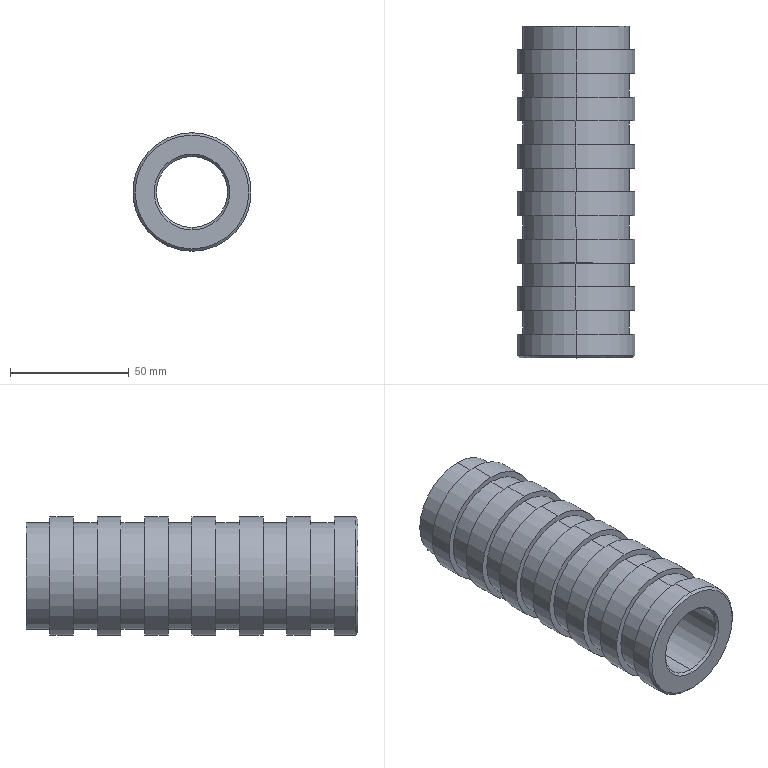Part | SolidWorks | features Revolution 1 | 1 solid | 49 faces | box 50 x 140 x 50 mm | volume 149689 mm3 | cylinder 30 | plane 15 | cone 4 | commonest cylinder face diameters 45 x14 50 x14 30 x2
STEP:
#1=CARTESIAN_POINT('',(0.,-230.,25.));
#2=VERTEX_POINT('',#1);
#3=CARTESIAN_POINT('',(0.,-230.,-25.));
#4=VERTEX_POINT('',#3);
#5=CARTESIAN_POINT('',(0.,-230.,0.));
#6=DIRECTION('',(0.,1.,0.));
#7=DIRECTION('',(0.,0.,1.));
#8=AXIS2_PLACEMENT_3D('',#5,#6,#7);
#9=CIRCLE('',#8,25.);
#10=EDGE_CURVE('',#2,#4,#9,.T.);
#11=ORIENTED_EDGE('',*,*,#10,.T.);
#12=CARTESIAN_POINT('',(0.,-220.,-25.));
#13=VERTEX_POINT('',#12);
#14=CARTESIAN_POINT('',(0.,-290.,-25.));
#15=DIRECTION('',(0.,1.,0.));
#16=VECTOR('',#15,1000.);
#17=LINE('',#14,#16);
#18=EDGE_CURVE('',#4,#13,#17,.T.);
#19=ORIENTED_EDGE('',*,*,#18,.T.);
#20=CARTESIAN_POINT('',(0.,-220.,25.));
#21=VERTEX_POINT('',#20);
#22=CARTESIAN_POINT('',(0.,-220.,0.));
#23=DIRECTION('',(0.,1.,0.));
#24=DIRECTION('',(0.,0.,1.));
#25=AXIS2_PLACEMENT_3D('',#22,#23,#24);
#26=CIRCLE('',#25,25.);
#27=EDGE_CURVE('',#21,#13,#26,.T.);
#28=ORIENTED_EDGE('',*,*,#27,.F.);
#29=CARTESIAN_POINT('',(0.,-290.,25.));
#30=DIRECTION('',(0.,1.,0.));
#31=VECTOR('',#30,1000.);
#32=LINE('',#29,#31);
#33=EDGE_CURVE('',#2,#21,#32,.T.);
#34=ORIENTED_EDGE('',*,*,#33,.F.);
#35=EDGE_LOOP('',(#11,#19,#28,#34));
#36=FACE_OUTER_BOUND('',#35,.T.);
#37=CARTESIAN_POINT('',(0.,-290.,0.));
#38=DIRECTION('',(0.,1.,0.));
#39=DIRECTION('',(0.,0.,1.));
#40=AXIS2_PLACEMENT_3D('',#37,#38,#39);
#41=CYLINDRICAL_SURFACE('',#40,25.);
#42=ADVANCED_FACE('',(#36),#41,.T.);
#43=CARTESIAN_POINT('',(0.,-240.,22.5));
#44=VERTEX_POINT('',#43);
#45=CARTESIAN_POINT('',(0.,-240.,-22.5));
#46=VERTEX_POINT('',#45);
#47=CARTESIAN_POINT('',(0.,-240.,0.));
#48=DIRECTION('',(0.,1.,0.));
#49=DIRECTION('',(0.,0.,1.));
#50=AXIS2_PLACEMENT_3D('',#47,#48,#49);
#51=CIRCLE('',#50,22.5);
#52=EDGE_CURVE('',#44,#46,#51,.T.);
#53=ORIENTED_EDGE('',*,*,#52,.T.);
#54=CARTESIAN_POINT('',(0.,-230.,-22.5));
#55=VERTEX_POINT('',#54);
#56=CARTESIAN_POINT('',(0.,-290.,-22.5));
#57=DIRECTION('',(0.,1.,0.));
#58=VECTOR('',#57,1000.);
#59=LINE('',#56,#58);
#60=EDGE_CURVE('',#46,#55,#59,.T.);
#61=ORIENTED_EDGE('',*,*,#60,.T.);
#62=CARTESIAN_POINT('',(0.,-230.,22.5));
#63=VERTEX_POINT('',#62);
#64=CARTESIAN_POINT('',(0.,-230.,0.));
#65=DIRECTION('',(0.,1.,0.));
#66=DIRECTION('',(0.,0.,1.));
#67=AXIS2_PLACEMENT_3D('',#64,#65,#66);
#68=CIRCLE('',#67,22.5);
#69=EDGE_CURVE('',#63,#55,#68,.T.);
#70=ORIENTED_EDGE('',*,*,#69,.F.);
#71=CARTESIAN_POINT('',(0.,-290.,22.5));
#72=DIRECTION('',(0.,1.,0.));
#73=VECTOR('',#72,1000.);
#74=LINE('',#71,#73);
#75=EDGE_CURVE('',#44,#63,#74,.T.);
#76=ORIENTED_EDGE('',*,*,#75,.F.);
#77=EDGE_LOOP('',(#53,#61,#70,#76));
#78=FACE_OUTER_BOUND('',#77,.T.);
#79=CARTESIAN_POINT('',(0.,-290.,0.));
#80=DIRECTION('',(0.,1.,0.));
#81=DIRECTION('',(0.,0.,1.));
#82=AXIS2_PLACEMENT_3D('',#79,#80,#81);
#83=CYLINDRICAL_SURFACE('',#82,22.5);
#84=ADVANCED_FACE('',(#78),#83,.T.);
#85=CARTESIAN_POINT('',(0.,-250.,25.));
#86=VERTEX_POINT('',#85);
#87=CARTESIAN_POINT('',(0.,-250.,-25.));
#88=VERTEX_POINT('',#87);
#89=CARTESIAN_POINT('',(0.,-250.,0.));
#90=DIRECTION('',(0.,1.,0.));
#91=DIRECTION('',(0.,0.,1.));
#92=AXIS2_PLACEMENT_3D('',#89,#90,#91);
#93=CIRCLE('',#92,25.);
#94=EDGE_CURVE('',#86,#88,#93,.T.);
#95=ORIENTED_EDGE('',*,*,#94,.T.);
#96=CARTESIAN_POINT('',(0.,-240.,-25.));
#97=VERTEX_POINT('',#96);
#98=CARTESIAN_POINT('',(0.,-290.,-25.));
#99=DIRECTION('',(0.,1.,0.));
#100=VECTOR('',#99,1000.);
#101=LINE('',#98,#100);
#102=EDGE_CURVE('',#88,#97,#101,.T.);
#103=ORIENTED_EDGE('',*,*,#102,.T.);
#104=CARTESIAN_POINT('',(0.,-240.,25.));
#105=VERTEX_POINT('',#104);
#106=CARTESIAN_POINT('',(0.,-240.,0.));
#107=DIRECTION('',(0.,1.,0.));
#108=DIRECTION('',(0.,0.,1.));
#109=AXIS2_PLACEMENT_3D('',#106,#107,#108);
#110=CIRCLE('',#109,25.);
#111=EDGE_CURVE('',#105,#97,#110,.T.);
#112=ORIENTED_EDGE('',*,*,#111,.F.);
#113=CARTESIAN_POINT('',(0.,-290.,25.));
#114=DIRECTION('',(0.,1.,0.));
#115=VECTOR('',#114,1000.);
#116=LINE('',#113,#115);
#117=EDGE_CURVE('',#86,#105,#116,.T.);
#118=ORIENTED_EDGE('',*,*,#117,.F.);
#119=EDGE_LOOP('',(#95,#103,#112,#118));
#120=FACE_OUTER_BOUND('',#119,.T.);
#121=CARTESIAN_POINT('',(0.,-290.,0.));
#122=DIRECTION('',(0.,1.,0.));
#123=DIRECTION('',(0.,0.,1.));
#124=AXIS2_PLACEMENT_3D('',#121,#122,#123);
#125=CYLINDRICAL_SURFACE('',#124,25.);
#126=ADVANCED_FACE('',(#120),#125,.T.);
#127=CARTESIAN_POINT('',(0.,-260.,22.5));
#128=VERTEX_POINT('',#127);
#129=CARTESIAN_POINT('',(0.,-260.,-22.5));
#130=VERTEX_POINT('',#129);
#131=CARTESIAN_POINT('',(0.,-260.,0.));
#132=DIRECTION('',(0.,1.,0.));
#133=DIRECTION('',(0.,0.,1.));
#134=AXIS2_PLACEMENT_3D('',#131,#132,#133);
#135=CIRCLE('',#134,22.5);
#136=EDGE_CURVE('',#128,#130,#135,.T.);
#137=ORIENTED_EDGE('',*,*,#136,.T.);
#138=CARTESIAN_POINT('',(0.,-250.,-22.5));
#139=VERTEX_POINT('',#138);
#140=CARTESIAN_POINT('',(0.,-290.,-22.5));
#141=DIRECTION('',(0.,1.,0.));
#142=VECTOR('',#141,1000.);
#143=LINE('',#140,#142);
#144=EDGE_CURVE('',#130,#139,#143,.T.);
#145=ORIENTED_EDGE('',*,*,#144,.T.);
#146=CARTESIAN_POINT('',(0.,-250.,22.5));
#147=VERTEX_POINT('',#146);
#148=CARTESIAN_POINT('',(0.,-250.,0.));
#149=DIRECTION('',(0.,1.,0.));
#150=DIRECTION('',(0.,0.,1.));
#151=AXIS2_PLACEMENT_3D('',#148,#149,#150);
#152=CIRCLE('',#151,22.5);
#153=EDGE_CURVE('',#147,#139,#152,.T.);
#154=ORIENTED_EDGE('',*,*,#153,.F.);
#155=CARTESIAN_POINT('',(0.,-290.,22.5));
#156=DIRECTION('',(0.,1.,0.));
#157=VECTOR('',#156,1000.);
#158=LINE('',#155,#157);
#159=EDGE_CURVE('',#128,#147,#158,.T.);
#160=ORIENTED_EDGE('',*,*,#159,.F.);
#161=EDGE_LOOP('',(#137,#145,#154,#160));
#162=FACE_OUTER_BOUND('',#161,.T.);
#163=CARTESIAN_POINT('',(0.,-290.,0.));
#164=DIRECTION('',(0.,1.,0.));
#165=DIRECTION('',(0.,0.,1.));
#166=AXIS2_PLACEMENT_3D('',#163,#164,#165);
#167=CYLINDRICAL_SURFACE('',#166,22.5);
#168=ADVANCED_FACE('',(#162),#167,.T.);
#169=CARTESIAN_POINT('',(0.,-270.,25.));
#170=VERTEX_POINT('',#169);
#171=CARTESIAN_POINT('',(0.,-270.,-25.));
#172=VERTEX_POINT('',#171);
#173=CARTESIAN_POINT('',(0.,-270.,0.));
#174=DIRECTION('',(0.,1.,0.));
#175=DIRECTION('',(0.,0.,1.));
#176=AXIS2_PLACEMENT_3D('',#173,#174,#175);
#177=CIRCLE('',#176,25.);
#178=EDGE_CURVE('',#170,#172,#177,.T.);
#179=ORIENTED_EDGE('',*,*,#178,.T.);
#180=CARTESIAN_POINT('',(0.,-260.,-25.));
#181=VERTEX_POINT('',#180);
#182=CARTESIAN_POINT('',(0.,-290.,-25.));
#183=DIRECTION('',(0.,1.,0.));
#184=VECTOR('',#183,1000.);
#185=LINE('',#182,#184);
#186=EDGE_CURVE('',#172,#181,#185,.T.);
#187=ORIENTED_EDGE('',*,*,#186,.T.);
#188=CARTESIAN_POINT('',(0.,-260.,25.));
#189=VERTEX_POINT('',#188);
#190=CARTESIAN_POINT('',(0.,-260.,0.));
#191=DIRECTION('',(0.,1.,0.));
#192=DIRECTION('',(0.,0.,1.));
#193=AXIS2_PLACEMENT_3D('',#190,#191,#192);
#194=CIRCLE('',#193,25.);
#195=EDGE_CURVE('',#189,#181,#194,.T.);
#196=ORIENTED_EDGE('',*,*,#195,.F.);
#197=CARTESIAN_POINT('',(0.,-290.,25.));
#198=DIRECTION('',(0.,1.,0.));
#199=VECTOR('',#198,1000.);
#200=LINE('',#197,#199);
#201=EDGE_CURVE('',#170,#189,#200,.T.);
#202=ORIENTED_EDGE('',*,*,#201,.F.);
#203=EDGE_LOOP('',(#179,#187,#196,#202));
#204=FACE_OUTER_BOUND('',#203,.T.);
#205=CARTESIAN_POINT('',(0.,-290.,0.));
#206=DIRECTION('',(0.,1.,0.));
#207=DIRECTION('',(0.,0.,1.));
#208=AXIS2_PLACEMENT_3D('',#205,#206,#207);
#209=CYLINDRICAL_SURFACE('',#208,25.);
#210=ADVANCED_FACE('',(#204),#209,.T.);
#211=CARTESIAN_POINT('',(0.,-280.,22.5));
#212=VERTEX_POINT('',#211);
#213=CARTESIAN_POINT('',(0.,-280.,-22.5));
#214=VERTEX_POINT('',#213);
#215=CARTESIAN_POINT('',(0.,-280.,0.));
#216=DIRECTION('',(0.,1.,0.));
#217=DIRECTION('',(0.,0.,1.));
#218=AXIS2_PLACEMENT_3D('',#215,#216,#217);
#219=CIRCLE('',#218,22.5);
#220=EDGE_CURVE('',#212,#214,#219,.T.);
#221=ORIENTED_EDGE('',*,*,#220,.T.);
#222=CARTESIAN_POINT('',(0.,-270.,-22.5));
#223=VERTEX_POINT('',#222);
#224=CARTESIAN_POINT('',(0.,-290.,-22.5));
#225=DIRECTION('',(0.,1.,0.));
#226=VECTOR('',#225,1000.);
#227=LINE('',#224,#226);
#228=EDGE_CURVE('',#214,#223,#227,.T.);
#229=ORIENTED_EDGE('',*,*,#228,.T.);
#230=CARTESIAN_POINT('',(0.,-270.,22.5));
#231=VERTEX_POINT('',#230);
#232=CARTESIAN_POINT('',(0.,-270.,0.));
#233=DIRECTION('',(0.,1.,0.));
#234=DIRECTION('',(0.,0.,1.));
#235=AXIS2_PLACEMENT_3D('',#232,#233,#234);
#236=CIRCLE('',#235,22.5);
#237=EDGE_CURVE('',#231,#223,#236,.T.);
#238=ORIENTED_EDGE('',*,*,#237,.F.);
#239=CARTESIAN_POINT('',(0.,-290.,22.5));
#240=DIRECTION('',(0.,1.,0.));
#241=VECTOR('',#240,1000.);
#242=LINE('',#239,#241);
#243=EDGE_CURVE('',#212,#231,#242,.T.);
#244=ORIENTED_EDGE('',*,*,#243,.F.);
#245=EDGE_LOOP('',(#221,#229,#238,#244));
#246=FACE_OUTER_BOUND('',#245,.T.);
#247=CARTESIAN_POINT('',(0.,-290.,0.));
#248=DIRECTION('',(0.,1.,0.));
#249=DIRECTION('',(0.,0.,1.));
#250=AXIS2_PLACEMENT_3D('',#247,#248,#249);
#251=CYLINDRICAL_SURFACE('',#250,22.5);
#252=ADVANCED_FACE('',(#246),#251,.T.);
#253=CARTESIAN_POINT('',(0.,-289.,25.));
#254=VERTEX_POINT('',#253);
#255=CARTESIAN_POINT('',(0.,-289.,-25.));
#256=VERTEX_POINT('',#255);
#257=CARTESIAN_POINT('',(0.,-289.,0.));
#258=DIRECTION('',(0.,1.,0.));
#259=DIRECTION('',(0.,0.,1.));
#260=AXIS2_PLACEMENT_3D('',#257,#258,#259);
#261=CIRCLE('',#260,25.);
#262=EDGE_CURVE('',#254,#256,#261,.T.);
#263=ORIENTED_EDGE('',*,*,#262,.T.);
#264=CARTESIAN_POINT('',(0.,-280.,-25.));
#265=VERTEX_POINT('',#264);
#266=CARTESIAN_POINT('',(0.,-290.,-25.));
#267=DIRECTION('',(0.,1.,0.));
#268=VECTOR('',#267,1000.);
#269=LINE('',#266,#268);
#270=EDGE_CURVE('',#256,#265,#269,.T.);
#271=ORIENTED_EDGE('',*,*,#270,.T.);
#272=CARTESIAN_POINT('',(0.,-280.,25.));
#273=VERTEX_POINT('',#272);
#274=CARTESIAN_POINT('',(0.,-280.,0.));
#275=DIRECTION('',(0.,1.,0.));
#276=DIRECTION('',(0.,0.,1.));
#277=AXIS2_PLACEMENT_3D('',#274,#275,#276);
#278=CIRCLE('',#277,25.);
#279=EDGE_CURVE('',#273,#265,#278,.T.);
#280=ORIENTED_EDGE('',*,*,#279,.F.);
#281=CARTESIAN_POINT('',(0.,-290.,25.));
#282=DIRECTION('',(0.,1.,0.));
#283=VECTOR('',#282,1000.);
#284=LINE('',#281,#283);
#285=EDGE_CURVE('',#254,#273,#284,.T.);
#286=ORIENTED_EDGE('',*,*,#285,.F.);
#287=EDGE_LOOP('',(#263,#271,#280,#286));
#288=FACE_OUTER_BOUND('',#287,.T.);
#289=CARTESIAN_POINT('',(0.,-290.,0.));
#290=DIRECTION('',(0.,1.,0.));
#291=DIRECTION('',(0.,0.,1.));
#292=AXIS2_PLACEMENT_3D('',#289,#290,#291);
#293=CYLINDRICAL_SURFACE('',#292,25.);
#294=ADVANCED_FACE('',(#288),#293,.T.);
#295=CARTESIAN_POINT('',(0.,-290.,24.));
#296=VERTEX_POINT('',#295);
#297=CARTESIAN_POINT('',(0.,-290.,-24.));
#298=VERTEX_POINT('',#297);
#299=CARTESIAN_POINT('',(0.,-290.,0.));
#300=DIRECTION('',(0.,1.,0.));
#301=DIRECTION('',(0.,0.,1.));
#302=AXIS2_PLACEMENT_3D('',#299,#300,#301);
#303=CIRCLE('',#302,24.);
#304=EDGE_CURVE('',#296,#298,#303,.T.);
#305=ORIENTED_EDGE('',*,*,#304,.T.);
#306=CARTESIAN_POINT('',(0.,-289.,-25.));
#307=DIRECTION('',(0.,0.7071,-0.7071));
#308=VECTOR('',#307,1000.);
#309=LINE('',#306,#308);
#310=EDGE_CURVE('',#298,#256,#309,.T.);
#311=ORIENTED_EDGE('',*,*,#310,.T.);
#312=ORIENTED_EDGE('',*,*,#262,.F.);
#313=CARTESIAN_POINT('',(0.,-289.,25.));
#314=DIRECTION('',(0.,0.7071,0.7071));
#315=VECTOR('',#314,1000.);
#316=LINE('',#313,#315);
#317=EDGE_CURVE('',#296,#254,#316,.T.);
#318=ORIENTED_EDGE('',*,*,#317,.F.);
#319=EDGE_LOOP('',(#305,#311,#312,#318));
#320=FACE_OUTER_BOUND('',#319,.T.);
#321=CARTESIAN_POINT('',(0.,-289.,0.));
#322=DIRECTION('',(0.,1.,0.));
#323=DIRECTION('',(0.,0.,1.));
#324=AXIS2_PLACEMENT_3D('',#321,#322,#323);
#325=CONICAL_SURFACE('',#324,25.,0.7854);
#326=ADVANCED_FACE('',(#320),#325,.T.);
#327=CARTESIAN_POINT('',(0.,-289.,-15.));
#328=VERTEX_POINT('',#327);
#329=CARTESIAN_POINT('',(0.,-289.,15.));
#330=VERTEX_POINT('',#329);
#331=CARTESIAN_POINT('',(0.,-289.,0.));
#332=DIRECTION('',(0.,1.,0.));
#333=DIRECTION('',(0.,0.,1.));
#334=AXIS2_PLACEMENT_3D('',#331,#332,#333);
#335=CIRCLE('',#334,15.);
#336=EDGE_CURVE('',#328,#330,#335,.T.);
#337=ORIENTED_EDGE('',*,*,#336,.T.);
#338=CARTESIAN_POINT('',(0.,-290.,16.));
#339=VERTEX_POINT('',#338);
#340=CARTESIAN_POINT('',(0.,-290.,16.));
#341=DIRECTION('',(0.,-0.7071,0.7071));
#342=VECTOR('',#341,1000.);
#343=LINE('',#340,#342);
#344=EDGE_CURVE('',#330,#339,#343,.T.);
#345=ORIENTED_EDGE('',*,*,#344,.T.);
#346=CARTESIAN_POINT('',(0.,-290.,-16.));
#347=VERTEX_POINT('',#346);
#348=CARTESIAN_POINT('',(0.,-290.,0.));
#349=DIRECTION('',(0.,1.,0.));
#350=DIRECTION('',(0.,0.,1.));
#351=AXIS2_PLACEMENT_3D('',#348,#349,#350);
#352=CIRCLE('',#351,16.);
#353=EDGE_CURVE('',#347,#339,#352,.T.);
#354=ORIENTED_EDGE('',*,*,#353,.F.);
#355=CARTESIAN_POINT('',(0.,-290.,-16.));
#356=DIRECTION('',(0.,-0.7071,-0.7071));
#357=VECTOR('',#356,1000.);
#358=LINE('',#355,#357);
#359=EDGE_CURVE('',#328,#347,#358,.T.);
#360=ORIENTED_EDGE('',*,*,#359,.F.);
#361=EDGE_LOOP('',(#337,#345,#354,#360));
#362=FACE_OUTER_BOUND('',#361,.T.);
#363=CARTESIAN_POINT('',(0.,-290.,0.));
#364=DIRECTION('',(0.,-1.,0.));
#365=DIRECTION('',(0.,0.,-1.));
#366=AXIS2_PLACEMENT_3D('',#363,#364,#365);
#367=CONICAL_SURFACE('',#366,16.,0.7854);
#368=ADVANCED_FACE('',(#362),#367,.F.);
#369=ORIENTED_EDGE('',*,*,#336,.F.);
#370=CARTESIAN_POINT('',(0.,-150.,-15.));
#371=VERTEX_POINT('',#370);
#372=CARTESIAN_POINT('',(0.,-290.,-15.));
#373=DIRECTION('',(0.,1.,0.));
#374=VECTOR('',#373,1000.);
#375=LINE('',#372,#374);
#376=EDGE_CURVE('',#328,#371,#375,.T.);
#377=ORIENTED_EDGE('',*,*,#376,.T.);
#378=CARTESIAN_POINT('',(0.,-150.,15.));
#379=VERTEX_POINT('',#378);
#380=CARTESIAN_POINT('',(0.,-150.,0.));
#381=DIRECTION('',(0.,1.,0.));
#382=DIRECTION('',(0.,0.,1.));
#383=AXIS2_PLACEMENT_3D('',#380,#381,#382);
#384=CIRCLE('',#383,15.);
#385=EDGE_CURVE('',#371,#379,#384,.T.);
#386=ORIENTED_EDGE('',*,*,#385,.T.);
#387=CARTESIAN_POINT('',(0.,-290.,15.));
#388=DIRECTION('',(0.,1.,0.));
#389=VECTOR('',#388,1000.);
#390=LINE('',#387,#389);
#391=EDGE_CURVE('',#330,#379,#390,.T.);
#392=ORIENTED_EDGE('',*,*,#391,.F.);
#393=EDGE_LOOP('',(#369,#377,#386,#392));
#394=FACE_OUTER_BOUND('',#393,.T.);
#395=CARTESIAN_POINT('',(0.,-290.,0.));
#396=DIRECTION('',(0.,1.,0.));
#397=DIRECTION('',(0.,0.,1.));
#398=AXIS2_PLACEMENT_3D('',#395,#396,#397);
#399=CYLINDRICAL_SURFACE('',#398,15.);
#400=ADVANCED_FACE('',(#394),#399,.F.);
#401=CARTESIAN_POINT('',(0.,-160.,22.5));
#402=VERTEX_POINT('',#401);
#403=CARTESIAN_POINT('',(0.,-160.,-22.5));
#404=VERTEX_POINT('',#403);
#405=CARTESIAN_POINT('',(0.,-160.,0.));
#406=DIRECTION('',(0.,1.,0.));
#407=DIRECTION('',(0.,0.,1.));
#408=AXIS2_PLACEMENT_3D('',#405,#406,#407);
#409=CIRCLE('',#408,22.5);
#410=EDGE_CURVE('',#402,#404,#409,.T.);
#411=ORIENTED_EDGE('',*,*,#410,.T.);
#412=CARTESIAN_POINT('',(0.,-150.,-22.5));
#413=VERTEX_POINT('',#412);
#414=CARTESIAN_POINT('',(0.,-290.,-22.5));
#415=DIRECTION('',(0.,1.,0.));
#416=VECTOR('',#415,1000.);
#417=LINE('',#414,#416);
#418=EDGE_CURVE('',#404,#413,#417,.T.);
#419=ORIENTED_EDGE('',*,*,#418,.T.);
#420=CARTESIAN_POINT('',(0.,-150.,22.5));
#421=VERTEX_POINT('',#420);
#422=CARTESIAN_POINT('',(0.,-150.,0.));
#423=DIRECTION('',(0.,1.,0.));
#424=DIRECTION('',(0.,0.,1.));
#425=AXIS2_PLACEMENT_3D('',#422,#423,#424);
#426=CIRCLE('',#425,22.5);
#427=EDGE_CURVE('',#421,#413,#426,.T.);
#428=ORIENTED_EDGE('',*,*,#427,.F.);
#429=CARTESIAN_POINT('',(0.,-290.,22.5));
#430=DIRECTION('',(0.,1.,0.));
#431=VECTOR('',#430,1000.);
#432=LINE('',#429,#431);
#433=EDGE_CURVE('',#402,#421,#432,.T.);
#434=ORIENTED_EDGE('',*,*,#433,.F.);
#435=EDGE_LOOP('',(#411,#419,#428,#434));
#436=FACE_OUTER_BOUND('',#435,.T.);
#437=CARTESIAN_POINT('',(0.,-290.,0.));
#438=DIRECTION('',(0.,1.,0.));
#439=DIRECTION('',(0.,0.,1.));
#440=AXIS2_PLACEMENT_3D('',#437,#438,#439);
#441=CYLINDRICAL_SURFACE('',#440,22.5);
#442=ADVANCED_FACE('',(#436),#441,.T.);
#443=CARTESIAN_POINT('',(0.,-170.,25.));
#444=VERTEX_POINT('',#443);
#445=CARTESIAN_POINT('',(0.,-170.,-25.));
#446=VERTEX_POINT('',#445);
#447=CARTESIAN_POINT('',(0.,-170.,0.));
#448=DIRECTION('',(0.,1.,0.));
#449=DIRECTION('',(0.,0.,1.));
#450=AXIS2_PLACEMENT_3D('',#447,#448,#449);
#451=CIRCLE('',#450,25.);
#452=EDGE_CURVE('',#444,#446,#451,.T.);
#453=ORIENTED_EDGE('',*,*,#452,.T.);
#454=CARTESIAN_POINT('',(0.,-160.,-25.));
#455=VERTEX_POINT('',#454);
#456=CARTESIAN_POINT('',(0.,-290.,-25.));
#457=DIRECTION('',(0.,1.,0.));
#458=VECTOR('',#457,1000.);
#459=LINE('',#456,#458);
#460=EDGE_CURVE('',#446,#455,#459,.T.);
#461=ORIENTED_EDGE('',*,*,#460,.T.);
#462=CARTESIAN_POINT('',(0.,-160.,25.));
#463=VERTEX_POINT('',#462);
#464=CARTESIAN_POINT('',(0.,-160.,0.));
#465=DIRECTION('',(0.,1.,0.));
#466=DIRECTION('',(0.,0.,1.));
#467=AXIS2_PLACEMENT_3D('',#464,#465,#466);
#468=CIRCLE('',#467,25.);
#469=EDGE_CURVE('',#463,#455,#468,.T.);
#470=ORIENTED_EDGE('',*,*,#469,.F.);
#471=CARTESIAN_POINT('',(0.,-290.,25.));
#472=DIRECTION('',(0.,1.,0.));
#473=VECTOR('',#472,1000.);
#474=LINE('',#471,#473);
#475=EDGE_CURVE('',#444,#463,#474,.T.);
#476=ORIENTED_EDGE('',*,*,#475,.F.);
#477=EDGE_LOOP('',(#453,#461,#470,#476));
#478=FACE_OUTER_BOUND('',#477,.T.);
#479=CARTESIAN_POINT('',(0.,-290.,0.));
#480=DIRECTION('',(0.,1.,0.));
#481=DIRECTION('',(0.,0.,1.));
#482=AXIS2_PLACEMENT_3D('',#479,#480,#481);
#483=CYLINDRICAL_SURFACE('',#482,25.);
#484=ADVANCED_FACE('',(#478),#483,.T.);
#485=CARTESIAN_POINT('',(0.,-180.,22.5));
#486=VERTEX_POINT('',#485);
#487=CARTESIAN_POINT('',(0.,-180.,-22.5));
#488=VERTEX_POINT('',#487);
#489=CARTESIAN_POINT('',(0.,-180.,0.));
#490=DIRECTION('',(0.,1.,0.));
#491=DIRECTION('',(0.,0.,1.));
#492=AXIS2_PLACEMENT_3D('',#489,#490,#491);
#493=CIRCLE('',#492,22.5);
#494=EDGE_CURVE('',#486,#488,#493,.T.);
#495=ORIENTED_EDGE('',*,*,#494,.T.);
#496=CARTESIAN_POINT('',(0.,-170.,-22.5));
#497=VERTEX_POINT('',#496);
#498=CARTESIAN_POINT('',(0.,-290.,-22.5));
#499=DIRECTION('',(0.,1.,0.));
#500=VECTOR('',#499,1000.);
#501=LINE('',#498,#500);
#502=EDGE_CURVE('',#488,#497,#501,.T.);
#503=ORIENTED_EDGE('',*,*,#502,.T.);
#504=CARTESIAN_POINT('',(0.,-170.,22.5));
#505=VERTEX_POINT('',#504);
#506=CARTESIAN_POINT('',(0.,-170.,0.));
#507=DIRECTION('',(0.,1.,0.));
#508=DIRECTION('',(0.,0.,1.));
#509=AXIS2_PLACEMENT_3D('',#506,#507,#508);
#510=CIRCLE('',#509,22.5);
#511=EDGE_CURVE('',#505,#497,#510,.T.);
#512=ORIENTED_EDGE('',*,*,#511,.F.);
#513=CARTESIAN_POINT('',(0.,-290.,22.5));
#514=DIRECTION('',(0.,1.,0.));
#515=VECTOR('',#514,1000.);
#516=LINE('',#513,#515);
#517=EDGE_CURVE('',#486,#505,#516,.T.);
#518=ORIENTED_EDGE('',*,*,#517,.F.);
#519=EDGE_LOOP('',(#495,#503,#512,#518));
#520=FACE_OUTER_BOUND('',#519,.T.);
#521=CARTESIAN_POINT('',(0.,-290.,0.));
#522=DIRECTION('',(0.,1.,0.));
#523=DIRECTION('',(0.,0.,1.));
#524=AXIS2_PLACEMENT_3D('',#521,#522,#523);
#525=CYLINDRICAL_SURFACE('',#524,22.5);
#526=ADVANCED_FACE('',(#520),#525,.T.);
#527=CARTESIAN_POINT('',(0.,-190.,25.));
#528=VERTEX_POINT('',#527);
#529=CARTESIAN_POINT('',(0.,-190.,-25.));
#530=VERTEX_POINT('',#529);
#531=CARTESIAN_POINT('',(0.,-190.,0.));
#532=DIRECTION('',(0.,1.,0.));
#533=DIRECTION('',(0.,0.,1.));
#534=AXIS2_PLACEMENT_3D('',#531,#532,#533);
#535=CIRCLE('',#534,25.);
#536=EDGE_CURVE('',#528,#530,#535,.T.);
#537=ORIENTED_EDGE('',*,*,#536,.T.);
#538=CARTESIAN_POINT('',(0.,-180.,-25.));
#539=VERTEX_POINT('',#538);
#540=CARTESIAN_POINT('',(0.,-290.,-25.));
#541=DIRECTION('',(0.,1.,0.));
#542=VECTOR('',#541,1000.);
#543=LINE('',#540,#542);
#544=EDGE_CURVE('',#530,#539,#543,.T.);
#545=ORIENTED_EDGE('',*,*,#544,.T.);
#546=CARTESIAN_POINT('',(0.,-180.,25.));
#547=VERTEX_POINT('',#546);
#548=CARTESIAN_POINT('',(0.,-180.,0.));
#549=DIRECTION('',(0.,1.,0.));
#550=DIRECTION('',(0.,0.,1.));
#551=AXIS2_PLACEMENT_3D('',#548,#549,#550);
#552=CIRCLE('',#551,25.);
#553=EDGE_CURVE('',#547,#539,#552,.T.);
#554=ORIENTED_EDGE('',*,*,#553,.F.);
#555=CARTESIAN_POINT('',(0.,-290.,25.));
#556=DIRECTION('',(0.,1.,0.));
#557=VECTOR('',#556,1000.);
#558=LINE('',#555,#557);
#559=EDGE_CURVE('',#528,#547,#558,.T.);
#560=ORIENTED_EDGE('',*,*,#559,.F.);
#561=EDGE_LOOP('',(#537,#545,#554,#560));
#562=FACE_OUTER_BOUND('',#561,.T.);
#563=CARTESIAN_POINT('',(0.,-290.,0.));
#564=DIRECTION('',(0.,1.,0.));
#565=DIRECTION('',(0.,0.,1.));
#566=AXIS2_PLACEMENT_3D('',#563,#564,#565);
#567=CYLINDRICAL_SURFACE('',#566,25.);
#568=ADVANCED_FACE('',(#562),#567,.T.);
#569=CARTESIAN_POINT('',(0.,-200.,22.5));
#570=VERTEX_POINT('',#569);
#571=CARTESIAN_POINT('',(0.,-200.,-22.5));
#572=VERTEX_POINT('',#571);
#573=CARTESIAN_POINT('',(0.,-200.,0.));
#574=DIRECTION('',(0.,1.,0.));
#575=DIRECTION('',(0.,0.,1.));
#576=AXIS2_PLACEMENT_3D('',#573,#574,#575);
#577=CIRCLE('',#576,22.5);
#578=EDGE_CURVE('',#570,#572,#577,.T.);
#579=ORIENTED_EDGE('',*,*,#578,.T.);
#580=CARTESIAN_POINT('',(0.,-190.,-22.5));
#581=VERTEX_POINT('',#580);
#582=CARTESIAN_POINT('',(0.,-290.,-22.5));
#583=DIRECTION('',(0.,1.,0.));
#584=VECTOR('',#583,1000.);
#585=LINE('',#582,#584);
#586=EDGE_CURVE('',#572,#581,#585,.T.);
#587=ORIENTED_EDGE('',*,*,#586,.T.);
#588=CARTESIAN_POINT('',(0.,-190.,22.5));
#589=VERTEX_POINT('',#588);
#590=CARTESIAN_POINT('',(0.,-190.,0.));
#591=DIRECTION('',(0.,1.,0.));
#592=DIRECTION('',(0.,0.,1.));
#593=AXIS2_PLACEMENT_3D('',#590,#591,#592);
#594=CIRCLE('',#593,22.5);
#595=EDGE_CURVE('',#589,#581,#594,.T.);
#596=ORIENTED_EDGE('',*,*,#595,.F.);
#597=CARTESIAN_POINT('',(0.,-290.,22.5));
#598=DIRECTION('',(0.,1.,0.));
#599=VECTOR('',#598,1000.);
#600=LINE('',#597,#599);
#601=EDGE_CURVE('',#570,#589,#600,.T.);
#602=ORIENTED_EDGE('',*,*,#601,.F.);
#603=EDGE_LOOP('',(#579,#587,#596,#602));
#604=FACE_OUTER_BOUND('',#603,.T.);
#605=CARTESIAN_POINT('',(0.,-290.,0.));
#606=DIRECTION('',(0.,1.,0.));
#607=DIRECTION('',(0.,0.,1.));
#608=AXIS2_PLACEMENT_3D('',#605,#606,#607);
#609=CYLINDRICAL_SURFACE('',#608,22.5);
#610=ADVANCED_FACE('',(#604),#609,.T.);
#611=CARTESIAN_POINT('',(0.,-210.,25.));
#612=VERTEX_POINT('',#611);
#613=CARTESIAN_POINT('',(0.,-210.,-25.));
#614=VERTEX_POINT('',#613);
#615=CARTESIAN_POINT('',(0.,-210.,0.));
#616=DIRECTION('',(0.,1.,0.));
#617=DIRECTION('',(0.,0.,1.));
#618=AXIS2_PLACEMENT_3D('',#615,#616,#617);
#619=CIRCLE('',#618,25.);
#620=EDGE_CURVE('',#612,#614,#619,.T.);
#621=ORIENTED_EDGE('',*,*,#620,.T.);
#622=CARTESIAN_POINT('',(0.,-200.,-25.));
#623=VERTEX_POINT('',#622);
#624=CARTESIAN_POINT('',(0.,-290.,-25.));
#625=DIRECTION('',(0.,1.,0.));
#626=VECTOR('',#625,1000.);
#627=LINE('',#624,#626);
#628=EDGE_CURVE('',#614,#623,#627,.T.);
#629=ORIENTED_EDGE('',*,*,#628,.T.);
#630=CARTESIAN_POINT('',(0.,-200.,25.));
#631=VERTEX_POINT('',#630);
#632=CARTESIAN_POINT('',(0.,-200.,0.));
#633=DIRECTION('',(0.,1.,0.));
#634=DIRECTION('',(0.,0.,1.));
#635=AXIS2_PLACEMENT_3D('',#632,#633,#634);
#636=CIRCLE('',#635,25.);
#637=EDGE_CURVE('',#631,#623,#636,.T.);
#638=ORIENTED_EDGE('',*,*,#637,.F.);
#639=CARTESIAN_POINT('',(0.,-290.,25.));
#640=DIRECTION('',(0.,1.,0.));
#641=VECTOR('',#640,1000.);
#642=LINE('',#639,#641);
#643=EDGE_CURVE('',#612,#631,#642,.T.);
#644=ORIENTED_EDGE('',*,*,#643,.F.);
#645=EDGE_LOOP('',(#621,#629,#638,#644));
#646=FACE_OUTER_BOUND('',#645,.T.);
#647=CARTESIAN_POINT('',(0.,-290.,0.));
#648=DIRECTION('',(0.,1.,0.));
#649=DIRECTION('',(0.,0.,1.));
#650=AXIS2_PLACEMENT_3D('',#647,#648,#649);
#651=CYLINDRICAL_SURFACE('',#650,25.);
#652=ADVANCED_FACE('',(#646),#651,.T.);
#653=CARTESIAN_POINT('',(0.,-220.,22.5));
#654=VERTEX_POINT('',#653);
#655=CARTESIAN_POINT('',(0.,-220.,-22.5));
#656=VERTEX_POINT('',#655);
#657=CARTESIAN_POINT('',(0.,-220.,0.));
#658=DIRECTION('',(0.,1.,0.));
#659=DIRECTION('',(0.,0.,1.));
#660=AXIS2_PLACEMENT_3D('',#657,#658,#659);
#661=CIRCLE('',#660,22.5);
#662=EDGE_CURVE('',#654,#656,#661,.T.);
#663=ORIENTED_EDGE('',*,*,#662,.T.);
#664=CARTESIAN_POINT('',(0.,-210.,-22.5));
#665=VERTEX_POINT('',#664);
#666=CARTESIAN_POINT('',(0.,-290.,-22.5));
#667=DIRECTION('',(0.,1.,0.));
#668=VECTOR('',#667,1000.);
#669=LINE('',#666,#668);
#670=EDGE_CURVE('',#656,#665,#669,.T.);
#671=ORIENTED_EDGE('',*,*,#670,.T.);
#672=CARTESIAN_POINT('',(0.,-210.,22.5));
#673=VERTEX_POINT('',#672);
#674=CARTESIAN_POINT('',(0.,-210.,0.));
#675=DIRECTION('',(0.,1.,0.));
#676=DIRECTION('',(0.,0.,1.));
#677=AXIS2_PLACEMENT_3D('',#674,#675,#676);
#678=CIRCLE('',#677,22.5);
#679=EDGE_CURVE('',#673,#665,#678,.T.);
#680=ORIENTED_EDGE('',*,*,#679,.F.);
#681=CARTESIAN_POINT('',(0.,-290.,22.5));
#682=DIRECTION('',(0.,1.,0.));
#683=VECTOR('',#682,1000.);
#684=LINE('',#681,#683);
#685=EDGE_CURVE('',#654,#673,#684,.T.);
#686=ORIENTED_EDGE('',*,*,#685,.F.);
#687=EDGE_LOOP('',(#663,#671,#680,#686));
#688=FACE_OUTER_BOUND('',#687,.T.);
#689=CARTESIAN_POINT('',(0.,-290.,0.));
#690=DIRECTION('',(0.,1.,0.));
#691=DIRECTION('',(0.,0.,1.));
#692=AXIS2_PLACEMENT_3D('',#689,#690,#691);
#693=CYLINDRICAL_SURFACE('',#692,22.5);
#694=ADVANCED_FACE('',(#688),#693,.T.);
#695=ORIENTED_EDGE('',*,*,#670,.F.);
#696=CARTESIAN_POINT('',(0.,-220.,0.));
#697=DIRECTION('',(0.,1.,0.));
#698=DIRECTION('',(0.,0.,1.));
#699=AXIS2_PLACEMENT_3D('',#696,#697,#698);
#700=CIRCLE('',#699,22.5);
#701=EDGE_CURVE('',#656,#654,#700,.T.);
#702=ORIENTED_EDGE('',*,*,#701,.T.);
#703=ORIENTED_EDGE('',*,*,#685,.T.);
#704=CARTESIAN_POINT('',(0.,-210.,0.));
#705=DIRECTION('',(0.,1.,0.));
#706=DIRECTION('',(0.,0.,1.));
#707=AXIS2_PLACEMENT_3D('',#704,#705,#706);
#708=CIRCLE('',#707,22.5);
#709=EDGE_CURVE('',#665,#673,#708,.T.);
#710=ORIENTED_EDGE('',*,*,#709,.F.);
#711=EDGE_LOOP('',(#695,#702,#703,#710));
#712=FACE_OUTER_BOUND('',#711,.T.);
#713=CARTESIAN_POINT('',(0.,-290.,0.));
#714=DIRECTION('',(0.,1.,0.));
#715=DIRECTION('',(0.,0.,1.));
#716=AXIS2_PLACEMENT_3D('',#713,#714,#715);
#717=CYLINDRICAL_SURFACE('',#716,22.5);
#718=ADVANCED_FACE('',(#712),#717,.T.);
#719=ORIENTED_EDGE('',*,*,#679,.T.);
#720=ORIENTED_EDGE('',*,*,#709,.T.);
#721=EDGE_LOOP('',(#719,#720));
#722=FACE_BOUND('',#721,.T.);
#723=ORIENTED_EDGE('',*,*,#620,.F.);
#724=CARTESIAN_POINT('',(0.,-210.,0.));
#725=DIRECTION('',(0.,1.,0.));
#726=DIRECTION('',(0.,0.,1.));
#727=AXIS2_PLACEMENT_3D('',#724,#725,#726);
#728=CIRCLE('',#727,25.);
#729=EDGE_CURVE('',#614,#612,#728,.T.);
#730=ORIENTED_EDGE('',*,*,#729,.F.);
#731=EDGE_LOOP('',(#723,#730));
#732=FACE_OUTER_BOUND('',#731,.T.);
#733=CARTESIAN_POINT('',(25.,-210.,0.));
#734=DIRECTION('',(0.,-1.,0.));
#735=DIRECTION('',(0.,0.,-1.));
#736=AXIS2_PLACEMENT_3D('',#733,#734,#735);
#737=PLANE('',#736);
#738=ADVANCED_FACE('',(#722,#732),#737,.T.);
#739=ORIENTED_EDGE('',*,*,#628,.F.);
#740=ORIENTED_EDGE('',*,*,#729,.T.);
#741=ORIENTED_EDGE('',*,*,#643,.T.);
#742=CARTESIAN_POINT('',(0.,-200.,0.));
#743=DIRECTION('',(0.,1.,0.));
#744=DIRECTION('',(0.,0.,1.));
#745=AXIS2_PLACEMENT_3D('',#742,#743,#744);
#746=CIRCLE('',#745,25.);
#747=EDGE_CURVE('',#623,#631,#746,.T.);
#748=ORIENTED_EDGE('',*,*,#747,.F.);
#749=EDGE_LOOP('',(#739,#740,#741,#748));
#750=FACE_OUTER_BOUND('',#749,.T.);
#751=CARTESIAN_POINT('',(0.,-290.,0.));
#752=DIRECTION('',(0.,1.,0.));
#753=DIRECTION('',(0.,0.,1.));
#754=AXIS2_PLACEMENT_3D('',#751,#752,#753);
#755=CYLINDRICAL_SURFACE('',#754,25.);
#756=ADVANCED_FACE('',(#750),#755,.T.);
#757=ORIENTED_EDGE('',*,*,#637,.T.);
#758=ORIENTED_EDGE('',*,*,#747,.T.);
#759=EDGE_LOOP('',(#757,#758));
#760=FACE_OUTER_BOUND('',#759,.T.);
#761=ORIENTED_EDGE('',*,*,#578,.F.);
#762=CARTESIAN_POINT('',(0.,-200.,0.));
#763=DIRECTION('',(0.,1.,0.));
#764=DIRECTION('',(0.,0.,1.));
#765=AXIS2_PLACEMENT_3D('',#762,#763,#764);
#766=CIRCLE('',#765,22.5);
#767=EDGE_CURVE('',#572,#570,#766,.T.);
#768=ORIENTED_EDGE('',*,*,#767,.F.);
#769=EDGE_LOOP('',(#761,#768));
#770=FACE_BOUND('',#769,.T.);
#771=CARTESIAN_POINT('',(22.5,-200.,0.));
#772=DIRECTION('',(0.,1.,0.));
#773=DIRECTION('',(0.,0.,1.));
#774=AXIS2_PLACEMENT_3D('',#771,#772,#773);
#775=PLANE('',#774);
#776=ADVANCED_FACE('',(#760,#770),#775,.T.);
#777=ORIENTED_EDGE('',*,*,#586,.F.);
#778=ORIENTED_EDGE('',*,*,#767,.T.);
#779=ORIENTED_EDGE('',*,*,#601,.T.);
#780=CARTESIAN_POINT('',(0.,-190.,0.));
#781=DIRECTION('',(0.,1.,0.));
#782=DIRECTION('',(0.,0.,1.));
#783=AXIS2_PLACEMENT_3D('',#780,#781,#782);
#784=CIRCLE('',#783,22.5);
#785=EDGE_CURVE('',#581,#589,#784,.T.);
#786=ORIENTED_EDGE('',*,*,#785,.F.);
#787=EDGE_LOOP('',(#777,#778,#779,#786));
#788=FACE_OUTER_BOUND('',#787,.T.);
#789=CARTESIAN_POINT('',(0.,-290.,0.));
#790=DIRECTION('',(0.,1.,0.));
#791=DIRECTION('',(0.,0.,1.));
#792=AXIS2_PLACEMENT_3D('',#789,#790,#791);
#793=CYLINDRICAL_SURFACE('',#792,22.5);
#794=ADVANCED_FACE('',(#788),#793,.T.);
#795=ORIENTED_EDGE('',*,*,#595,.T.);
#796=ORIENTED_EDGE('',*,*,#785,.T.);
#797=EDGE_LOOP('',(#795,#796));
#798=FACE_BOUND('',#797,.T.);
#799=ORIENTED_EDGE('',*,*,#536,.F.);
#800=CARTESIAN_POINT('',(0.,-190.,0.));
#801=DIRECTION('',(0.,1.,0.));
#802=DIRECTION('',(0.,0.,1.));
#803=AXIS2_PLACEMENT_3D('',#800,#801,#802);
#804=CIRCLE('',#803,25.);
#805=EDGE_CURVE('',#530,#528,#804,.T.);
#806=ORIENTED_EDGE('',*,*,#805,.F.);
#807=EDGE_LOOP('',(#799,#806));
#808=FACE_OUTER_BOUND('',#807,.T.);
#809=CARTESIAN_POINT('',(25.,-190.,0.));
#810=DIRECTION('',(0.,-1.,0.));
#811=DIRECTION('',(0.,0.,-1.));
#812=AXIS2_PLACEMENT_3D('',#809,#810,#811);
#813=PLANE('',#812);
#814=ADVANCED_FACE('',(#798,#808),#813,.T.);
#815=ORIENTED_EDGE('',*,*,#544,.F.);
#816=ORIENTED_EDGE('',*,*,#805,.T.);
#817=ORIENTED_EDGE('',*,*,#559,.T.);
#818=CARTESIAN_POINT('',(0.,-180.,0.));
#819=DIRECTION('',(0.,1.,0.));
#820=DIRECTION('',(0.,0.,1.));
#821=AXIS2_PLACEMENT_3D('',#818,#819,#820);
#822=CIRCLE('',#821,25.);
#823=EDGE_CURVE('',#539,#547,#822,.T.);
#824=ORIENTED_EDGE('',*,*,#823,.F.);
#825=EDGE_LOOP('',(#815,#816,#817,#824));
#826=FACE_OUTER_BOUND('',#825,.T.);
#827=CARTESIAN_POINT('',(0.,-290.,0.));
#828=DIRECTION('',(0.,1.,0.));
#829=DIRECTION('',(0.,0.,1.));
#830=AXIS2_PLACEMENT_3D('',#827,#828,#829);
#831=CYLINDRICAL_SURFACE('',#830,25.);
#832=ADVANCED_FACE('',(#826),#831,.T.);
#833=ORIENTED_EDGE('',*,*,#553,.T.);
#834=ORIENTED_EDGE('',*,*,#823,.T.);
#835=EDGE_LOOP('',(#833,#834));
#836=FACE_OUTER_BOUND('',#835,.T.);
#837=ORIENTED_EDGE('',*,*,#494,.F.);
#838=CARTESIAN_POINT('',(0.,-180.,0.));
#839=DIRECTION('',(0.,1.,0.));
#840=DIRECTION('',(0.,0.,1.));
#841=AXIS2_PLACEMENT_3D('',#838,#839,#840);
#842=CIRCLE('',#841,22.5);
#843=EDGE_CURVE('',#488,#486,#842,.T.);
#844=ORIENTED_EDGE('',*,*,#843,.F.);
#845=EDGE_LOOP('',(#837,#844));
#846=FACE_BOUND('',#845,.T.);
#847=CARTESIAN_POINT('',(22.5,-180.,0.));
#848=DIRECTION('',(0.,1.,0.));
#849=DIRECTION('',(0.,0.,1.));
#850=AXIS2_PLACEMENT_3D('',#847,#848,#849);
#851=PLANE('',#850);
#852=ADVANCED_FACE('',(#836,#846),#851,.T.);
#853=ORIENTED_EDGE('',*,*,#502,.F.);
#854=ORIENTED_EDGE('',*,*,#843,.T.);
#855=ORIENTED_EDGE('',*,*,#517,.T.);
#856=CARTESIAN_POINT('',(0.,-170.,0.));
#857=DIRECTION('',(0.,1.,0.));
#858=DIRECTION('',(0.,0.,1.));
#859=AXIS2_PLACEMENT_3D('',#856,#857,#858);
#860=CIRCLE('',#859,22.5);
#861=EDGE_CURVE('',#497,#505,#860,.T.);
#862=ORIENTED_EDGE('',*,*,#861,.F.);
#863=EDGE_LOOP('',(#853,#854,#855,#862));
#864=FACE_OUTER_BOUND('',#863,.T.);
#865=CARTESIAN_POINT('',(0.,-290.,0.));
#866=DIRECTION('',(0.,1.,0.));
#867=DIRECTION('',(0.,0.,1.));
#868=AXIS2_PLACEMENT_3D('',#865,#866,#867);
#869=CYLINDRICAL_SURFACE('',#868,22.5);
#870=ADVANCED_FACE('',(#864),#869,.T.);
#871=ORIENTED_EDGE('',*,*,#511,.T.);
#872=ORIENTED_EDGE('',*,*,#861,.T.);
#873=EDGE_LOOP('',(#871,#872));
#874=FACE_BOUND('',#873,.T.);
#875=ORIENTED_EDGE('',*,*,#452,.F.);
#876=CARTESIAN_POINT('',(0.,-170.,0.));
#877=DIRECTION('',(0.,1.,0.));
#878=DIRECTION('',(0.,0.,1.));
#879=AXIS2_PLACEMENT_3D('',#876,#877,#878);
#880=CIRCLE('',#879,25.);
#881=EDGE_CURVE('',#446,#444,#880,.T.);
#882=ORIENTED_EDGE('',*,*,#881,.F.);
#883=EDGE_LOOP('',(#875,#882));
#884=FACE_OUTER_BOUND('',#883,.T.);
#885=CARTESIAN_POINT('',(25.,-170.,0.));
#886=DIRECTION('',(0.,-1.,0.));
#887=DIRECTION('',(0.,0.,-1.));
#888=AXIS2_PLACEMENT_3D('',#885,#886,#887);
#889=PLANE('',#888);
#890=ADVANCED_FACE('',(#874,#884),#889,.T.);
#891=ORIENTED_EDGE('',*,*,#460,.F.);
#892=ORIENTED_EDGE('',*,*,#881,.T.);
#893=ORIENTED_EDGE('',*,*,#475,.T.);
#894=CARTESIAN_POINT('',(0.,-160.,0.));
#895=DIRECTION('',(0.,1.,0.));
#896=DIRECTION('',(0.,0.,1.));
#897=AXIS2_PLACEMENT_3D('',#894,#895,#896);
#898=CIRCLE('',#897,25.);
#899=EDGE_CURVE('',#455,#463,#898,.T.);
#900=ORIENTED_EDGE('',*,*,#899,.F.);
#901=EDGE_LOOP('',(#891,#892,#893,#900));
#902=FACE_OUTER_BOUND('',#901,.T.);
#903=CARTESIAN_POINT('',(0.,-290.,0.));
#904=DIRECTION('',(0.,1.,0.));
#905=DIRECTION('',(0.,0.,1.));
#906=AXIS2_PLACEMENT_3D('',#903,#904,#905);
#907=CYLINDRICAL_SURFACE('',#906,25.);
#908=ADVANCED_FACE('',(#902),#907,.T.);
#909=ORIENTED_EDGE('',*,*,#469,.T.);
#910=ORIENTED_EDGE('',*,*,#899,.T.);
#911=EDGE_LOOP('',(#909,#910));
#912=FACE_OUTER_BOUND('',#911,.T.);
#913=ORIENTED_EDGE('',*,*,#410,.F.);
#914=CARTESIAN_POINT('',(0.,-160.,0.));
#915=DIRECTION('',(0.,1.,0.));
#916=DIRECTION('',(0.,0.,1.));
#917=AXIS2_PLACEMENT_3D('',#914,#915,#916);
#918=CIRCLE('',#917,22.5);
#919=EDGE_CURVE('',#404,#402,#918,.T.);
#920=ORIENTED_EDGE('',*,*,#919,.F.);
#921=EDGE_LOOP('',(#913,#920));
#922=FACE_BOUND('',#921,.T.);
#923=CARTESIAN_POINT('',(22.5,-160.,0.));
#924=DIRECTION('',(0.,1.,0.));
#925=DIRECTION('',(0.,0.,1.));
#926=AXIS2_PLACEMENT_3D('',#923,#924,#925);
#927=PLANE('',#926);
#928=ADVANCED_FACE('',(#912,#922),#927,.T.);
#929=ORIENTED_EDGE('',*,*,#418,.F.);
#930=ORIENTED_EDGE('',*,*,#919,.T.);
#931=ORIENTED_EDGE('',*,*,#433,.T.);
#932=CARTESIAN_POINT('',(0.,-150.,0.));
#933=DIRECTION('',(0.,1.,0.));
#934=DIRECTION('',(0.,0.,1.));
#935=AXIS2_PLACEMENT_3D('',#932,#933,#934);
#936=CIRCLE('',#935,22.5);
#937=EDGE_CURVE('',#413,#421,#936,.T.);
#938=ORIENTED_EDGE('',*,*,#937,.F.);
#939=EDGE_LOOP('',(#929,#930,#931,#938));
#940=FACE_OUTER_BOUND('',#939,.T.);
#941=CARTESIAN_POINT('',(0.,-290.,0.));
#942=DIRECTION('',(0.,1.,0.));
#943=DIRECTION('',(0.,0.,1.));
#944=AXIS2_PLACEMENT_3D('',#941,#942,#943);
#945=CYLINDRICAL_SURFACE('',#944,22.5);
#946=ADVANCED_FACE('',(#940),#945,.T.);
#947=ORIENTED_EDGE('',*,*,#427,.T.);
#948=ORIENTED_EDGE('',*,*,#937,.T.);
#949=EDGE_LOOP('',(#947,#948));
#950=FACE_OUTER_BOUND('',#949,.T.);
#951=CARTESIAN_POINT('',(0.,-150.,0.));
#952=DIRECTION('',(0.,1.,0.));
#953=DIRECTION('',(0.,0.,1.));
#954=AXIS2_PLACEMENT_3D('',#951,#952,#953);
#955=CIRCLE('',#954,15.);
#956=EDGE_CURVE('',#379,#371,#955,.T.);
#957=ORIENTED_EDGE('',*,*,#956,.F.);
#958=ORIENTED_EDGE('',*,*,#385,.F.);
#959=EDGE_LOOP('',(#957,#958));
#960=FACE_BOUND('',#959,.T.);
#961=CARTESIAN_POINT('',(15.,-150.,0.));
#962=DIRECTION('',(0.,1.,0.));
#963=DIRECTION('',(0.,0.,1.));
#964=AXIS2_PLACEMENT_3D('',#961,#962,#963);
#965=PLANE('',#964);
#966=ADVANCED_FACE('',(#950,#960),#965,.T.);
#967=ORIENTED_EDGE('',*,*,#376,.F.);
#968=CARTESIAN_POINT('',(0.,-289.,0.));
#969=DIRECTION('',(0.,1.,0.));
#970=DIRECTION('',(0.,0.,1.));
#971=AXIS2_PLACEMENT_3D('',#968,#969,#970);
#972=CIRCLE('',#971,15.);
#973=EDGE_CURVE('',#330,#328,#972,.T.);
#974=ORIENTED_EDGE('',*,*,#973,.F.);
#975=ORIENTED_EDGE('',*,*,#391,.T.);
#976=ORIENTED_EDGE('',*,*,#956,.T.);
#977=EDGE_LOOP('',(#967,#974,#975,#976));
#978=FACE_OUTER_BOUND('',#977,.T.);
#979=CARTESIAN_POINT('',(0.,-290.,0.));
#980=DIRECTION('',(0.,1.,0.));
#981=DIRECTION('',(0.,0.,1.));
#982=AXIS2_PLACEMENT_3D('',#979,#980,#981);
#983=CYLINDRICAL_SURFACE('',#982,15.);
#984=ADVANCED_FACE('',(#978),#983,.F.);
#985=ORIENTED_EDGE('',*,*,#344,.F.);
#986=ORIENTED_EDGE('',*,*,#973,.T.);
#987=ORIENTED_EDGE('',*,*,#359,.T.);
#988=CARTESIAN_POINT('',(0.,-290.,0.));
#989=DIRECTION('',(0.,1.,0.));
#990=DIRECTION('',(0.,0.,1.));
#991=AXIS2_PLACEMENT_3D('',#988,#989,#990);
#992=CIRCLE('',#991,16.);
#993=EDGE_CURVE('',#339,#347,#992,.T.);
#994=ORIENTED_EDGE('',*,*,#993,.F.);
#995=EDGE_LOOP('',(#985,#986,#987,#994));
#996=FACE_OUTER_BOUND('',#995,.T.);
#997=CARTESIAN_POINT('',(0.,-290.,0.));
#998=DIRECTION('',(0.,-1.,0.));
#999=DIRECTION('',(0.,0.,-1.));
#1000=AXIS2_PLACEMENT_3D('',#997,#998,#999);
#1001=CONICAL_SURFACE('',#1000,16.,0.7854);
#1002=ADVANCED_FACE('',(#996),#1001,.F.);
#1003=ORIENTED_EDGE('',*,*,#353,.T.);
#1004=ORIENTED_EDGE('',*,*,#993,.T.);
#1005=EDGE_LOOP('',(#1003,#1004));
#1006=FACE_BOUND('',#1005,.T.);
#1007=ORIENTED_EDGE('',*,*,#304,.F.);
#1008=CARTESIAN_POINT('',(0.,-290.,0.));
#1009=DIRECTION('',(0.,1.,0.));
#1010=DIRECTION('',(0.,0.,1.));
#1011=AXIS2_PLACEMENT_3D('',#1008,#1009,#1010);
#1012=CIRCLE('',#1011,24.);
#1013=EDGE_CURVE('',#298,#296,#1012,.T.);
#1014=ORIENTED_EDGE('',*,*,#1013,.F.);
#1015=EDGE_LOOP('',(#1007,#1014));
#1016=FACE_OUTER_BOUND('',#1015,.T.);
#1017=CARTESIAN_POINT('',(24.,-290.,0.));
#1018=DIRECTION('',(0.,-1.,0.));
#1019=DIRECTION('',(0.,0.,-1.));
#1020=AXIS2_PLACEMENT_3D('',#1017,#1018,#1019);
#1021=PLANE('',#1020);
#1022=ADVANCED_FACE('',(#1006,#1016),#1021,.T.);
#1023=ORIENTED_EDGE('',*,*,#310,.F.);
#1024=ORIENTED_EDGE('',*,*,#1013,.T.);
#1025=ORIENTED_EDGE('',*,*,#317,.T.);
#1026=CARTESIAN_POINT('',(0.,-289.,0.));
#1027=DIRECTION('',(0.,1.,0.));
#1028=DIRECTION('',(0.,0.,1.));
#1029=AXIS2_PLACEMENT_3D('',#1026,#1027,#1028);
#1030=CIRCLE('',#1029,25.);
#1031=EDGE_CURVE('',#256,#254,#1030,.T.);
#1032=ORIENTED_EDGE('',*,*,#1031,.F.);
#1033=EDGE_LOOP('',(#1023,#1024,#1025,#1032));
#1034=FACE_OUTER_BOUND('',#1033,.T.);
#1035=CARTESIAN_POINT('',(0.,-289.,0.));
#1036=DIRECTION('',(0.,1.,0.));
#1037=DIRECTION('',(0.,0.,1.));
#1038=AXIS2_PLACEMENT_3D('',#1035,#1036,#1037);
#1039=CONICAL_SURFACE('',#1038,25.,0.7854);
#1040=ADVANCED_FACE('',(#1034),#1039,.T.);
#1041=ORIENTED_EDGE('',*,*,#270,.F.);
#1042=ORIENTED_EDGE('',*,*,#1031,.T.);
#1043=ORIENTED_EDGE('',*,*,#285,.T.);
#1044=CARTESIAN_POINT('',(0.,-280.,0.));
#1045=DIRECTION('',(0.,1.,0.));
#1046=DIRECTION('',(0.,0.,1.));
#1047=AXIS2_PLACEMENT_3D('',#1044,#1045,#1046);
#1048=CIRCLE('',#1047,25.);
#1049=EDGE_CURVE('',#265,#273,#1048,.T.);
#1050=ORIENTED_EDGE('',*,*,#1049,.F.);
#1051=EDGE_LOOP('',(#1041,#1042,#1043,#1050));
#1052=FACE_OUTER_BOUND('',#1051,.T.);
#1053=CARTESIAN_POINT('',(0.,-290.,0.));
#1054=DIRECTION('',(0.,1.,0.));
#1055=DIRECTION('',(0.,0.,1.));
#1056=AXIS2_PLACEMENT_3D('',#1053,#1054,#1055);
#1057=CYLINDRICAL_SURFACE('',#1056,25.);
#1058=ADVANCED_FACE('',(#1052),#1057,.T.);
#1059=ORIENTED_EDGE('',*,*,#279,.T.);
#1060=ORIENTED_EDGE('',*,*,#1049,.T.);
#1061=EDGE_LOOP('',(#1059,#1060));
#1062=FACE_OUTER_BOUND('',#1061,.T.);
#1063=ORIENTED_EDGE('',*,*,#220,.F.);
#1064=CARTESIAN_POINT('',(0.,-280.,0.));
#1065=DIRECTION('',(0.,1.,0.));
#1066=DIRECTION('',(0.,0.,1.));
#1067=AXIS2_PLACEMENT_3D('',#1064,#1065,#1066);
#1068=CIRCLE('',#1067,22.5);
#1069=EDGE_CURVE('',#214,#212,#1068,.T.);
#1070=ORIENTED_EDGE('',*,*,#1069,.F.);
#1071=EDGE_LOOP('',(#1063,#1070));
#1072=FACE_BOUND('',#1071,.T.);
#1073=CARTESIAN_POINT('',(22.5,-280.,0.));
#1074=DIRECTION('',(0.,1.,0.));
#1075=DIRECTION('',(0.,0.,1.));
#1076=AXIS2_PLACEMENT_3D('',#1073,#1074,#1075);
#1077=PLANE('',#1076);
#1078=ADVANCED_FACE('',(#1062,#1072),#1077,.T.);
#1079=ORIENTED_EDGE('',*,*,#228,.F.);
#1080=ORIENTED_EDGE('',*,*,#1069,.T.);
#1081=ORIENTED_EDGE('',*,*,#243,.T.);
#1082=CARTESIAN_POINT('',(0.,-270.,0.));
#1083=DIRECTION('',(0.,1.,0.));
#1084=DIRECTION('',(0.,0.,1.));
#1085=AXIS2_PLACEMENT_3D('',#1082,#1083,#1084);
#1086=CIRCLE('',#1085,22.5);
#1087=EDGE_CURVE('',#223,#231,#1086,.T.);
#1088=ORIENTED_EDGE('',*,*,#1087,.F.);
#1089=EDGE_LOOP('',(#1079,#1080,#1081,#1088));
#1090=FACE_OUTER_BOUND('',#1089,.T.);
#1091=CARTESIAN_POINT('',(0.,-290.,0.));
#1092=DIRECTION('',(0.,1.,0.));
#1093=DIRECTION('',(0.,0.,1.));
#1094=AXIS2_PLACEMENT_3D('',#1091,#1092,#1093);
#1095=CYLINDRICAL_SURFACE('',#1094,22.5);
#1096=ADVANCED_FACE('',(#1090),#1095,.T.);
#1097=ORIENTED_EDGE('',*,*,#237,.T.);
#1098=ORIENTED_EDGE('',*,*,#1087,.T.);
#1099=EDGE_LOOP('',(#1097,#1098));
#1100=FACE_BOUND('',#1099,.T.);
#1101=ORIENTED_EDGE('',*,*,#178,.F.);
#1102=CARTESIAN_POINT('',(0.,-270.,0.));
#1103=DIRECTION('',(0.,1.,0.));
#1104=DIRECTION('',(0.,0.,1.));
#1105=AXIS2_PLACEMENT_3D('',#1102,#1103,#1104);
#1106=CIRCLE('',#1105,25.);
#1107=EDGE_CURVE('',#172,#170,#1106,.T.);
#1108=ORIENTED_EDGE('',*,*,#1107,.F.);
#1109=EDGE_LOOP('',(#1101,#1108));
#1110=FACE_OUTER_BOUND('',#1109,.T.);
#1111=CARTESIAN_POINT('',(25.,-270.,0.));
#1112=DIRECTION('',(0.,-1.,0.));
#1113=DIRECTION('',(0.,0.,-1.));
#1114=AXIS2_PLACEMENT_3D('',#1111,#1112,#1113);
#1115=PLANE('',#1114);
#1116=ADVANCED_FACE('',(#1100,#1110),#1115,.T.);
#1117=ORIENTED_EDGE('',*,*,#186,.F.);
#1118=ORIENTED_EDGE('',*,*,#1107,.T.);
#1119=ORIENTED_EDGE('',*,*,#201,.T.);
#1120=CARTESIAN_POINT('',(0.,-260.,0.));
#1121=DIRECTION('',(0.,1.,0.));
#1122=DIRECTION('',(0.,0.,1.));
#1123=AXIS2_PLACEMENT_3D('',#1120,#1121,#1122);
#1124=CIRCLE('',#1123,25.);
#1125=EDGE_CURVE('',#181,#189,#1124,.T.);
#1126=ORIENTED_EDGE('',*,*,#1125,.F.);
#1127=EDGE_LOOP('',(#1117,#1118,#1119,#1126));
#1128=FACE_OUTER_BOUND('',#1127,.T.);
#1129=CARTESIAN_POINT('',(0.,-290.,0.));
#1130=DIRECTION('',(0.,1.,0.));
#1131=DIRECTION('',(0.,0.,1.));
#1132=AXIS2_PLACEMENT_3D('',#1129,#1130,#1131);
#1133=CYLINDRICAL_SURFACE('',#1132,25.);
#1134=ADVANCED_FACE('',(#1128),#1133,.T.);
#1135=ORIENTED_EDGE('',*,*,#195,.T.);
#1136=ORIENTED_EDGE('',*,*,#1125,.T.);
#1137=EDGE_LOOP('',(#1135,#1136));
#1138=FACE_OUTER_BOUND('',#1137,.T.);
#1139=ORIENTED_EDGE('',*,*,#136,.F.);
#1140=CARTESIAN_POINT('',(0.,-260.,0.));
#1141=DIRECTION('',(0.,1.,0.));
#1142=DIRECTION('',(0.,0.,1.));
#1143=AXIS2_PLACEMENT_3D('',#1140,#1141,#1142);
#1144=CIRCLE('',#1143,22.5);
#1145=EDGE_CURVE('',#130,#128,#1144,.T.);
#1146=ORIENTED_EDGE('',*,*,#1145,.F.);
#1147=EDGE_LOOP('',(#1139,#1146));
#1148=FACE_BOUND('',#1147,.T.);
#1149=CARTESIAN_POINT('',(22.5,-260.,0.));
#1150=DIRECTION('',(0.,1.,0.));
#1151=DIRECTION('',(0.,0.,1.));
#1152=AXIS2_PLACEMENT_3D('',#1149,#1150,#1151);
#1153=PLANE('',#1152);
#1154=ADVANCED_FACE('',(#1138,#1148),#1153,.T.);
#1155=ORIENTED_EDGE('',*,*,#144,.F.);
#1156=ORIENTED_EDGE('',*,*,#1145,.T.);
#1157=ORIENTED_EDGE('',*,*,#159,.T.);
#1158=CARTESIAN_POINT('',(0.,-250.,0.));
#1159=DIRECTION('',(0.,1.,0.));
#1160=DIRECTION('',(0.,0.,1.));
#1161=AXIS2_PLACEMENT_3D('',#1158,#1159,#1160);
#1162=CIRCLE('',#1161,22.5);
#1163=EDGE_CURVE('',#139,#147,#1162,.T.);
#1164=ORIENTED_EDGE('',*,*,#1163,.F.);
#1165=EDGE_LOOP('',(#1155,#1156,#1157,#1164));
#1166=FACE_OUTER_BOUND('',#1165,.T.);
#1167=CARTESIAN_POINT('',(0.,-290.,0.));
#1168=DIRECTION('',(0.,1.,0.));
#1169=DIRECTION('',(0.,0.,1.));
#1170=AXIS2_PLACEMENT_3D('',#1167,#1168,#1169);
#1171=CYLINDRICAL_SURFACE('',#1170,22.5);
#1172=ADVANCED_FACE('',(#1166),#1171,.T.);
#1173=ORIENTED_EDGE('',*,*,#153,.T.);
#1174=ORIENTED_EDGE('',*,*,#1163,.T.);
#1175=EDGE_LOOP('',(#1173,#1174));
#1176=FACE_BOUND('',#1175,.T.);
#1177=ORIENTED_EDGE('',*,*,#94,.F.);
#1178=CARTESIAN_POINT('',(0.,-250.,0.));
#1179=DIRECTION('',(0.,1.,0.));
#1180=DIRECTION('',(0.,0.,1.));
#1181=AXIS2_PLACEMENT_3D('',#1178,#1179,#1180);
#1182=CIRCLE('',#1181,25.);
#1183=EDGE_CURVE('',#88,#86,#1182,.T.);
#1184=ORIENTED_EDGE('',*,*,#1183,.F.);
#1185=EDGE_LOOP('',(#1177,#1184));
#1186=FACE_OUTER_BOUND('',#1185,.T.);
#1187=CARTESIAN_POINT('',(25.,-250.,0.));
#1188=DIRECTION('',(0.,-1.,0.));
#1189=DIRECTION('',(0.,0.,-1.));
#1190=AXIS2_PLACEMENT_3D('',#1187,#1188,#1189);
#1191=PLANE('',#1190);
#1192=ADVANCED_FACE('',(#1176,#1186),#1191,.T.);
#1193=ORIENTED_EDGE('',*,*,#102,.F.);
#1194=ORIENTED_EDGE('',*,*,#1183,.T.);
#1195=ORIENTED_EDGE('',*,*,#117,.T.);
#1196=CARTESIAN_POINT('',(0.,-240.,0.));
#1197=DIRECTION('',(0.,1.,0.));
#1198=DIRECTION('',(0.,0.,1.));
#1199=AXIS2_PLACEMENT_3D('',#1196,#1197,#1198);
#1200=CIRCLE('',#1199,25.);
#1201=EDGE_CURVE('',#97,#105,#1200,.T.);
#1202=ORIENTED_EDGE('',*,*,#1201,.F.);
#1203=EDGE_LOOP('',(#1193,#1194,#1195,#1202));
#1204=FACE_OUTER_BOUND('',#1203,.T.);
#1205=CARTESIAN_POINT('',(0.,-290.,0.));
#1206=DIRECTION('',(0.,1.,0.));
#1207=DIRECTION('',(0.,0.,1.));
#1208=AXIS2_PLACEMENT_3D('',#1205,#1206,#1207);
#1209=CYLINDRICAL_SURFACE('',#1208,25.);
#1210=ADVANCED_FACE('',(#1204),#1209,.T.);
#1211=ORIENTED_EDGE('',*,*,#111,.T.);
#1212=ORIENTED_EDGE('',*,*,#1201,.T.);
#1213=EDGE_LOOP('',(#1211,#1212));
#1214=FACE_OUTER_BOUND('',#1213,.T.);
#1215=ORIENTED_EDGE('',*,*,#52,.F.);
#1216=CARTESIAN_POINT('',(0.,-240.,0.));
#1217=DIRECTION('',(0.,1.,0.));
#1218=DIRECTION('',(0.,0.,1.));
#1219=AXIS2_PLACEMENT_3D('',#1216,#1217,#1218);
#1220=CIRCLE('',#1219,22.5);
#1221=EDGE_CURVE('',#46,#44,#1220,.T.);
#1222=ORIENTED_EDGE('',*,*,#1221,.F.);
#1223=EDGE_LOOP('',(#1215,#1222));
#1224=FACE_BOUND('',#1223,.T.);
#1225=CARTESIAN_POINT('',(22.5,-240.,0.));
#1226=DIRECTION('',(0.,1.,0.));
#1227=DIRECTION('',(0.,0.,1.));
#1228=AXIS2_PLACEMENT_3D('',#1225,#1226,#1227);
#1229=PLANE('',#1228);
#1230=ADVANCED_FACE('',(#1214,#1224),#1229,.T.);
#1231=ORIENTED_EDGE('',*,*,#60,.F.);
#1232=ORIENTED_EDGE('',*,*,#1221,.T.);
#1233=ORIENTED_EDGE('',*,*,#75,.T.);
#1234=CARTESIAN_POINT('',(0.,-230.,0.));
#1235=DIRECTION('',(0.,1.,0.));
#1236=DIRECTION('',(0.,0.,1.));
#1237=AXIS2_PLACEMENT_3D('',#1234,#1235,#1236);
#1238=CIRCLE('',#1237,22.5);
#1239=EDGE_CURVE('',#55,#63,#1238,.T.);
#1240=ORIENTED_EDGE('',*,*,#1239,.F.);
#1241=EDGE_LOOP('',(#1231,#1232,#1233,#1240));
#1242=FACE_OUTER_BOUND('',#1241,.T.);
#1243=CARTESIAN_POINT('',(0.,-290.,0.));
#1244=DIRECTION('',(0.,1.,0.));
#1245=DIRECTION('',(0.,0.,1.));
#1246=AXIS2_PLACEMENT_3D('',#1243,#1244,#1245);
#1247=CYLINDRICAL_SURFACE('',#1246,22.5);
#1248=ADVANCED_FACE('',(#1242),#1247,.T.);
#1249=ORIENTED_EDGE('',*,*,#69,.T.);
#1250=ORIENTED_EDGE('',*,*,#1239,.T.);
#1251=EDGE_LOOP('',(#1249,#1250));
#1252=FACE_BOUND('',#1251,.T.);
#1253=ORIENTED_EDGE('',*,*,#10,.F.);
#1254=CARTESIAN_POINT('',(0.,-230.,0.));
#1255=DIRECTION('',(0.,1.,0.));
#1256=DIRECTION('',(0.,0.,1.));
#1257=AXIS2_PLACEMENT_3D('',#1254,#1255,#1256);
#1258=CIRCLE('',#1257,25.);
#1259=EDGE_CURVE('',#4,#2,#1258,.T.);
#1260=ORIENTED_EDGE('',*,*,#1259,.F.);
#1261=EDGE_LOOP('',(#1253,#1260));
#1262=FACE_OUTER_BOUND('',#1261,.T.);
#1263=CARTESIAN_POINT('',(25.,-230.,0.));
#1264=DIRECTION('',(0.,-1.,0.));
#1265=DIRECTION('',(0.,0.,-1.));
#1266=AXIS2_PLACEMENT_3D('',#1263,#1264,#1265);
#1267=PLANE('',#1266);
#1268=ADVANCED_FACE('',(#1252,#1262),#1267,.T.);
#1269=ORIENTED_EDGE('',*,*,#18,.F.);
#1270=ORIENTED_EDGE('',*,*,#1259,.T.);
#1271=ORIENTED_EDGE('',*,*,#33,.T.);
#1272=CARTESIAN_POINT('',(0.,-220.,0.));
#1273=DIRECTION('',(0.,1.,0.));
#1274=DIRECTION('',(0.,0.,1.));
#1275=AXIS2_PLACEMENT_3D('',#1272,#1273,#1274);
#1276=CIRCLE('',#1275,25.);
#1277=EDGE_CURVE('',#13,#21,#1276,.T.);
#1278=ORIENTED_EDGE('',*,*,#1277,.F.);
#1279=EDGE_LOOP('',(#1269,#1270,#1271,#1278));
#1280=FACE_OUTER_BOUND('',#1279,.T.);
#1281=CARTESIAN_POINT('',(0.,-290.,0.));
#1282=DIRECTION('',(0.,1.,0.));
#1283=DIRECTION('',(0.,0.,1.));
#1284=AXIS2_PLACEMENT_3D('',#1281,#1282,#1283);
#1285=CYLINDRICAL_SURFACE('',#1284,25.);
#1286=ADVANCED_FACE('',(#1280),#1285,.T.);
#1287=ORIENTED_EDGE('',*,*,#27,.T.);
#1288=ORIENTED_EDGE('',*,*,#1277,.T.);
#1289=EDGE_LOOP('',(#1287,#1288));
#1290=FACE_OUTER_BOUND('',#1289,.T.);
#1291=ORIENTED_EDGE('',*,*,#662,.F.);
#1292=ORIENTED_EDGE('',*,*,#701,.F.);
#1293=EDGE_LOOP('',(#1291,#1292));
#1294=FACE_BOUND('',#1293,.T.);
#1295=CARTESIAN_POINT('',(22.5,-220.,0.));
#1296=DIRECTION('',(0.,1.,0.));
#1297=DIRECTION('',(0.,0.,1.));
#1298=AXIS2_PLACEMENT_3D('',#1295,#1296,#1297);
#1299=PLANE('',#1298);
#1300=ADVANCED_FACE('',(#1290,#1294),#1299,.T.);
#1301=CLOSED_SHELL('',(#42,#84,#126,#168,#210,#252,#294,#326,#368,#400,#442,#484,#526,#568,#610,#652,#694,#718,#738,#756,#776,#794,#814,#832,#852,#870,#890,#908,#928,#946,#966,#984,#1002,#1022,#1040,#1058,#1078,#1096,#1116,#1134,#1154,#1172,#1192,#1210,#1230,#1248,#1268,#1286,#1300));
#1302=MANIFOLD_SOLID_BREP('',#1301);
#1303=CARTESIAN_POINT('',(0.,0.,0.));
#1304=DIRECTION('',(0.,0.,1.));
#1305=DIRECTION('',(1.,0.,0.));
#1306=AXIS2_PLACEMENT_3D('',#1303,#1304,#1305);
#1307=(LENGTH_UNIT()NAMED_UNIT(*)SI_UNIT(.MILLI.,.METRE.));
#1308=UNCERTAINTY_MEASURE_WITH_UNIT(LENGTH_MEASURE(0.00001),#1307,'','');
#1309=(NAMED_UNIT(*)PLANE_ANGLE_UNIT()SI_UNIT($,.RADIAN.));
#1310=(NAMED_UNIT(*)SI_UNIT($,.STERADIAN.)SOLID_ANGLE_UNIT());
#1311=(GEOMETRIC_REPRESENTATION_CONTEXT(3)GLOBAL_UNCERTAINTY_ASSIGNED_CONTEXT((#1308))GLOBAL_UNIT_ASSIGNED_CONTEXT((#1307,#1309,#1310))REPRESENTATION_CONTEXT('',''));
#1312=ADVANCED_BREP_SHAPE_REPRESENTATION('',(#1302,#1306),#1311);